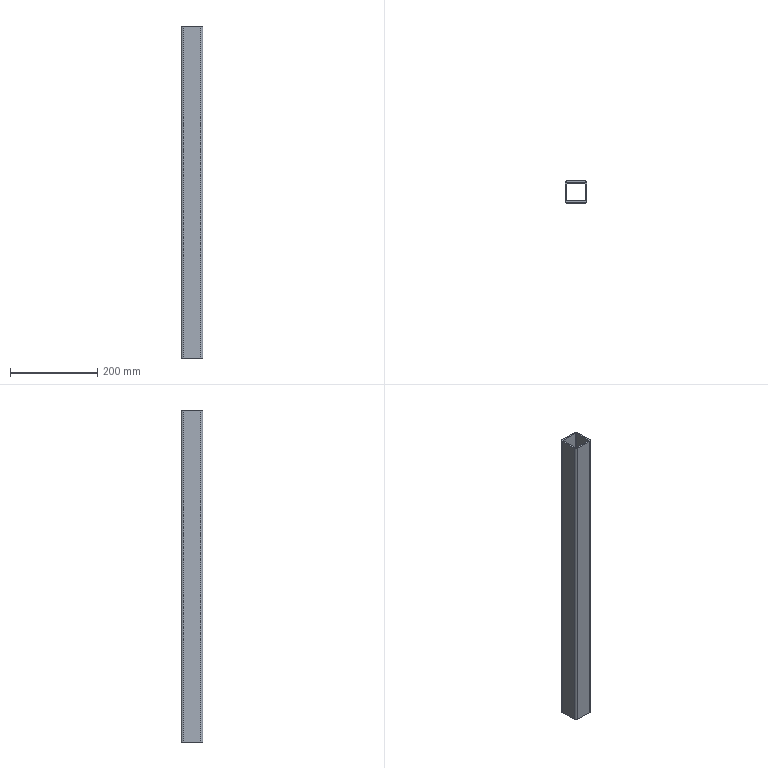Part | STEP file | 冲床-300配套压波_id1134_x_t | 1 solid | 18 faces | box 50 x 50 x 760 mm | volume 543703 mm3 | plane 10 | cylinder 8 | commonest cylinder face diameters 2 x4 10 x4
STEP:
#1=CARTESIAN_POINT('',(1164.,275.,-20.));
#2=VERTEX_POINT('',#1);
#3=CARTESIAN_POINT('',(1164.,235.,-20.));
#4=VERTEX_POINT('',#3);
#5=CARTESIAN_POINT('',(1164.,30.,-20.));
#6=DIRECTION('',(0.,-1.,0.));
#7=VECTOR('',#6,1.);
#8=LINE('',#5,#7);
#9=EDGE_CURVE('',#2,#4,#8,.T.);
#10=ORIENTED_EDGE('',*,*,#9,.F.);
#11=CARTESIAN_POINT('',(1165.,276.,-20.));
#12=VERTEX_POINT('',#11);
#13=CARTESIAN_POINT('',(1165.,275.,-20.));
#14=DIRECTION('',(0.,0.,1.));
#15=DIRECTION('',(1.,0.,0.));
#16=AXIS2_PLACEMENT_3D('',#13,#14,#15);
#17=CIRCLE('',#16,1.);
#18=EDGE_CURVE('',#12,#2,#17,.T.);
#19=ORIENTED_EDGE('',*,*,#18,.F.);
#20=CARTESIAN_POINT('',(1205.,276.,-20.));
#21=VERTEX_POINT('',#20);
#22=CARTESIAN_POINT('',(10.,276.,-20.));
#23=DIRECTION('',(-1.,0.,0.));
#24=VECTOR('',#23,1.);
#25=LINE('',#22,#24);
#26=EDGE_CURVE('',#21,#12,#25,.T.);
#27=ORIENTED_EDGE('',*,*,#26,.F.);
#28=CARTESIAN_POINT('',(1206.,275.,-20.));
#29=VERTEX_POINT('',#28);
#30=CARTESIAN_POINT('',(1205.,275.,-20.));
#31=DIRECTION('',(0.,0.,1.));
#32=DIRECTION('',(1.,0.,0.));
#33=AXIS2_PLACEMENT_3D('',#30,#31,#32);
#34=CIRCLE('',#33,1.);
#35=EDGE_CURVE('',#29,#21,#34,.T.);
#36=ORIENTED_EDGE('',*,*,#35,.F.);
#37=CARTESIAN_POINT('',(1206.,235.,-20.));
#38=VERTEX_POINT('',#37);
#39=CARTESIAN_POINT('',(1206.,30.,-20.));
#40=DIRECTION('',(0.,1.,0.));
#41=VECTOR('',#40,1.);
#42=LINE('',#39,#41);
#43=EDGE_CURVE('',#38,#29,#42,.T.);
#44=ORIENTED_EDGE('',*,*,#43,.F.);
#45=CARTESIAN_POINT('',(1205.,234.,-20.));
#46=VERTEX_POINT('',#45);
#47=CARTESIAN_POINT('',(1205.,235.,-20.));
#48=DIRECTION('',(0.,0.,1.));
#49=DIRECTION('',(1.,0.,0.));
#50=AXIS2_PLACEMENT_3D('',#47,#48,#49);
#51=CIRCLE('',#50,1.);
#52=EDGE_CURVE('',#46,#38,#51,.T.);
#53=ORIENTED_EDGE('',*,*,#52,.F.);
#54=CARTESIAN_POINT('',(1165.,234.,-20.));
#55=VERTEX_POINT('',#54);
#56=CARTESIAN_POINT('',(10.,234.,-20.));
#57=DIRECTION('',(1.,0.,0.));
#58=VECTOR('',#57,1.);
#59=LINE('',#56,#58);
#60=EDGE_CURVE('',#55,#46,#59,.T.);
#61=ORIENTED_EDGE('',*,*,#60,.F.);
#62=CARTESIAN_POINT('',(1165.,235.,-20.));
#63=DIRECTION('',(0.,0.,1.));
#64=DIRECTION('',(1.,0.,0.));
#65=AXIS2_PLACEMENT_3D('',#62,#63,#64);
#66=CIRCLE('',#65,1.);
#67=EDGE_CURVE('',#4,#55,#66,.T.);
#68=ORIENTED_EDGE('',*,*,#67,.F.);
#69=EDGE_LOOP('',(#10,#19,#27,#36,#44,#53,#61,#68));
#70=FACE_BOUND('',#69,.T.);
#71=CARTESIAN_POINT('',(1160.,275.,-20.));
#72=VERTEX_POINT('',#71);
#73=CARTESIAN_POINT('',(1160.,235.,-20.));
#74=VERTEX_POINT('',#73);
#75=CARTESIAN_POINT('',(1160.,275.,-20.));
#76=DIRECTION('',(0.,-1.,0.));
#77=VECTOR('',#76,1.);
#78=LINE('',#75,#77);
#79=EDGE_CURVE('',#72,#74,#78,.T.);
#80=ORIENTED_EDGE('',*,*,#79,.T.);
#81=CARTESIAN_POINT('',(1165.,230.,-20.));
#82=VERTEX_POINT('',#81);
#83=CARTESIAN_POINT('',(1165.,235.,-20.));
#84=DIRECTION('',(0.,0.,1.));
#85=DIRECTION('',(1.,0.,0.));
#86=AXIS2_PLACEMENT_3D('',#83,#84,#85);
#87=CIRCLE('',#86,5.);
#88=EDGE_CURVE('',#74,#82,#87,.T.);
#89=ORIENTED_EDGE('',*,*,#88,.T.);
#90=CARTESIAN_POINT('',(1205.,230.,-20.));
#91=VERTEX_POINT('',#90);
#92=CARTESIAN_POINT('',(1165.,230.,-20.));
#93=DIRECTION('',(1.,0.,0.));
#94=VECTOR('',#93,1.);
#95=LINE('',#92,#94);
#96=EDGE_CURVE('',#82,#91,#95,.T.);
#97=ORIENTED_EDGE('',*,*,#96,.T.);
#98=CARTESIAN_POINT('',(1210.,235.,-20.));
#99=VERTEX_POINT('',#98);
#100=CARTESIAN_POINT('',(1205.,235.,-20.));
#101=DIRECTION('',(0.,0.,1.));
#102=DIRECTION('',(1.,0.,0.));
#103=AXIS2_PLACEMENT_3D('',#100,#101,#102);
#104=CIRCLE('',#103,5.);
#105=EDGE_CURVE('',#91,#99,#104,.T.);
#106=ORIENTED_EDGE('',*,*,#105,.T.);
#107=CARTESIAN_POINT('',(1210.,275.,-20.));
#108=VERTEX_POINT('',#107);
#109=CARTESIAN_POINT('',(1210.,235.,-20.));
#110=DIRECTION('',(0.,1.,0.));
#111=VECTOR('',#110,1.);
#112=LINE('',#109,#111);
#113=EDGE_CURVE('',#99,#108,#112,.T.);
#114=ORIENTED_EDGE('',*,*,#113,.T.);
#115=CARTESIAN_POINT('',(1205.,280.,-20.));
#116=VERTEX_POINT('',#115);
#117=CARTESIAN_POINT('',(1205.,275.,-20.));
#118=DIRECTION('',(0.,0.,1.));
#119=DIRECTION('',(1.,0.,0.));
#120=AXIS2_PLACEMENT_3D('',#117,#118,#119);
#121=CIRCLE('',#120,5.);
#122=EDGE_CURVE('',#108,#116,#121,.T.);
#123=ORIENTED_EDGE('',*,*,#122,.T.);
#124=CARTESIAN_POINT('',(1165.,280.,-20.));
#125=VERTEX_POINT('',#124);
#126=CARTESIAN_POINT('',(1205.,280.,-20.));
#127=DIRECTION('',(-1.,0.,0.));
#128=VECTOR('',#127,1.);
#129=LINE('',#126,#128);
#130=EDGE_CURVE('',#116,#125,#129,.T.);
#131=ORIENTED_EDGE('',*,*,#130,.T.);
#132=CARTESIAN_POINT('',(1165.,275.,-20.));
#133=DIRECTION('',(0.,0.,1.));
#134=DIRECTION('',(1.,0.,0.));
#135=AXIS2_PLACEMENT_3D('',#132,#133,#134);
#136=CIRCLE('',#135,5.);
#137=EDGE_CURVE('',#125,#72,#136,.T.);
#138=ORIENTED_EDGE('',*,*,#137,.T.);
#139=EDGE_LOOP('',(#80,#89,#97,#106,#114,#123,#131,#138));
#140=FACE_BOUND('',#139,.T.);
#141=CARTESIAN_POINT('',(10.,30.,-20.));
#142=DIRECTION('',(0.,0.,1.));
#143=DIRECTION('',(1.,0.,0.));
#144=AXIS2_PLACEMENT_3D('',#141,#142,#143);
#145=PLANE('',#144);
#146=ADVANCED_FACE('',(#70,#140),#145,.T.);
#147=CARTESIAN_POINT('',(1165.,230.,-780.));
#148=VERTEX_POINT('',#147);
#149=CARTESIAN_POINT('',(1165.,230.,-740.));
#150=DIRECTION('',(0.,0.,1.));
#151=VECTOR('',#150,1.);
#152=LINE('',#149,#151);
#153=EDGE_CURVE('',#148,#82,#152,.T.);
#154=ORIENTED_EDGE('',*,*,#153,.T.);
#155=ORIENTED_EDGE('',*,*,#88,.F.);
#156=CARTESIAN_POINT('',(1160.,235.,-780.));
#157=VERTEX_POINT('',#156);
#158=CARTESIAN_POINT('',(1160.,235.,-740.));
#159=DIRECTION('',(0.,0.,1.));
#160=VECTOR('',#159,1.);
#161=LINE('',#158,#160);
#162=EDGE_CURVE('',#157,#74,#161,.T.);
#163=ORIENTED_EDGE('',*,*,#162,.F.);
#164=CARTESIAN_POINT('',(1165.,235.,-780.));
#165=DIRECTION('',(0.,0.,1.));
#166=DIRECTION('',(1.,0.,0.));
#167=AXIS2_PLACEMENT_3D('',#164,#165,#166);
#168=CIRCLE('',#167,5.);
#169=EDGE_CURVE('',#157,#148,#168,.T.);
#170=ORIENTED_EDGE('',*,*,#169,.T.);
#171=EDGE_LOOP('',(#154,#155,#163,#170));
#172=FACE_OUTER_BOUND('',#171,.T.);
#173=CARTESIAN_POINT('',(1165.,235.,-740.));
#174=DIRECTION('',(0.,0.,1.));
#175=DIRECTION('',(1.,0.,0.));
#176=AXIS2_PLACEMENT_3D('',#173,#174,#175);
#177=CYLINDRICAL_SURFACE('',#176,5.);
#178=ADVANCED_FACE('',(#172),#177,.T.);
#179=CARTESIAN_POINT('',(1205.,230.,-780.));
#180=VERTEX_POINT('',#179);
#181=CARTESIAN_POINT('',(1205.,230.,-740.));
#182=DIRECTION('',(0.,0.,1.));
#183=VECTOR('',#182,1.);
#184=LINE('',#181,#183);
#185=EDGE_CURVE('',#180,#91,#184,.T.);
#186=ORIENTED_EDGE('',*,*,#185,.T.);
#187=ORIENTED_EDGE('',*,*,#96,.F.);
#188=ORIENTED_EDGE('',*,*,#153,.F.);
#189=CARTESIAN_POINT('',(1165.,230.,-780.));
#190=DIRECTION('',(1.,0.,0.));
#191=VECTOR('',#190,1.);
#192=LINE('',#189,#191);
#193=EDGE_CURVE('',#148,#180,#192,.T.);
#194=ORIENTED_EDGE('',*,*,#193,.T.);
#195=EDGE_LOOP('',(#186,#187,#188,#194));
#196=FACE_OUTER_BOUND('',#195,.T.);
#197=CARTESIAN_POINT('',(1165.,230.,-740.));
#198=DIRECTION('',(0.,-1.,0.));
#199=DIRECTION('',(1.,0.,0.));
#200=AXIS2_PLACEMENT_3D('',#197,#198,#199);
#201=PLANE('',#200);
#202=ADVANCED_FACE('',(#196),#201,.T.);
#203=CARTESIAN_POINT('',(1210.,235.,-780.));
#204=VERTEX_POINT('',#203);
#205=CARTESIAN_POINT('',(1210.,235.,-740.));
#206=DIRECTION('',(0.,0.,1.));
#207=VECTOR('',#206,1.);
#208=LINE('',#205,#207);
#209=EDGE_CURVE('',#204,#99,#208,.T.);
#210=ORIENTED_EDGE('',*,*,#209,.T.);
#211=ORIENTED_EDGE('',*,*,#105,.F.);
#212=ORIENTED_EDGE('',*,*,#185,.F.);
#213=CARTESIAN_POINT('',(1205.,235.,-780.));
#214=DIRECTION('',(0.,0.,1.));
#215=DIRECTION('',(1.,0.,0.));
#216=AXIS2_PLACEMENT_3D('',#213,#214,#215);
#217=CIRCLE('',#216,5.);
#218=EDGE_CURVE('',#180,#204,#217,.T.);
#219=ORIENTED_EDGE('',*,*,#218,.T.);
#220=EDGE_LOOP('',(#210,#211,#212,#219));
#221=FACE_OUTER_BOUND('',#220,.T.);
#222=CARTESIAN_POINT('',(1205.,235.,-740.));
#223=DIRECTION('',(0.,0.,1.));
#224=DIRECTION('',(1.,0.,0.));
#225=AXIS2_PLACEMENT_3D('',#222,#223,#224);
#226=CYLINDRICAL_SURFACE('',#225,5.);
#227=ADVANCED_FACE('',(#221),#226,.T.);
#228=CARTESIAN_POINT('',(1210.,275.,-780.));
#229=VERTEX_POINT('',#228);
#230=CARTESIAN_POINT('',(1210.,275.,-740.));
#231=DIRECTION('',(0.,0.,1.));
#232=VECTOR('',#231,1.);
#233=LINE('',#230,#232);
#234=EDGE_CURVE('',#229,#108,#233,.T.);
#235=ORIENTED_EDGE('',*,*,#234,.T.);
#236=ORIENTED_EDGE('',*,*,#113,.F.);
#237=ORIENTED_EDGE('',*,*,#209,.F.);
#238=CARTESIAN_POINT('',(1210.,235.,-780.));
#239=DIRECTION('',(0.,1.,0.));
#240=VECTOR('',#239,1.);
#241=LINE('',#238,#240);
#242=EDGE_CURVE('',#204,#229,#241,.T.);
#243=ORIENTED_EDGE('',*,*,#242,.T.);
#244=EDGE_LOOP('',(#235,#236,#237,#243));
#245=FACE_OUTER_BOUND('',#244,.T.);
#246=CARTESIAN_POINT('',(1210.,235.,-740.));
#247=DIRECTION('',(1.,0.,0.));
#248=DIRECTION('',(0.,0.,-1.));
#249=AXIS2_PLACEMENT_3D('',#246,#247,#248);
#250=PLANE('',#249);
#251=ADVANCED_FACE('',(#245),#250,.T.);
#252=CARTESIAN_POINT('',(1205.,280.,-780.));
#253=VERTEX_POINT('',#252);
#254=CARTESIAN_POINT('',(1205.,280.,-740.));
#255=DIRECTION('',(0.,0.,1.));
#256=VECTOR('',#255,1.);
#257=LINE('',#254,#256);
#258=EDGE_CURVE('',#253,#116,#257,.T.);
#259=ORIENTED_EDGE('',*,*,#258,.T.);
#260=ORIENTED_EDGE('',*,*,#122,.F.);
#261=ORIENTED_EDGE('',*,*,#234,.F.);
#262=CARTESIAN_POINT('',(1205.,275.,-780.));
#263=DIRECTION('',(0.,0.,1.));
#264=DIRECTION('',(1.,0.,0.));
#265=AXIS2_PLACEMENT_3D('',#262,#263,#264);
#266=CIRCLE('',#265,5.);
#267=EDGE_CURVE('',#229,#253,#266,.T.);
#268=ORIENTED_EDGE('',*,*,#267,.T.);
#269=EDGE_LOOP('',(#259,#260,#261,#268));
#270=FACE_OUTER_BOUND('',#269,.T.);
#271=CARTESIAN_POINT('',(1205.,275.,-740.));
#272=DIRECTION('',(0.,0.,1.));
#273=DIRECTION('',(1.,0.,0.));
#274=AXIS2_PLACEMENT_3D('',#271,#272,#273);
#275=CYLINDRICAL_SURFACE('',#274,5.);
#276=ADVANCED_FACE('',(#270),#275,.T.);
#277=CARTESIAN_POINT('',(1165.,276.,-780.));
#278=VERTEX_POINT('',#277);
#279=CARTESIAN_POINT('',(1164.,275.,-780.));
#280=VERTEX_POINT('',#279);
#281=CARTESIAN_POINT('',(1165.,275.,-780.));
#282=DIRECTION('',(0.,0.,1.));
#283=DIRECTION('',(1.,0.,0.));
#284=AXIS2_PLACEMENT_3D('',#281,#282,#283);
#285=CIRCLE('',#284,1.);
#286=EDGE_CURVE('',#278,#280,#285,.T.);
#287=ORIENTED_EDGE('',*,*,#286,.T.);
#288=CARTESIAN_POINT('',(1164.,235.,-780.));
#289=VERTEX_POINT('',#288);
#290=CARTESIAN_POINT('',(1164.,235.,-780.));
#291=DIRECTION('',(0.,-1.,0.));
#292=VECTOR('',#291,1.);
#293=LINE('',#290,#292);
#294=EDGE_CURVE('',#280,#289,#293,.T.);
#295=ORIENTED_EDGE('',*,*,#294,.T.);
#296=CARTESIAN_POINT('',(1165.,234.,-780.));
#297=VERTEX_POINT('',#296);
#298=CARTESIAN_POINT('',(1165.,235.,-780.));
#299=DIRECTION('',(0.,0.,1.));
#300=DIRECTION('',(1.,0.,0.));
#301=AXIS2_PLACEMENT_3D('',#298,#299,#300);
#302=CIRCLE('',#301,1.);
#303=EDGE_CURVE('',#289,#297,#302,.T.);
#304=ORIENTED_EDGE('',*,*,#303,.T.);
#305=CARTESIAN_POINT('',(1205.,234.,-780.));
#306=VERTEX_POINT('',#305);
#307=CARTESIAN_POINT('',(1165.,234.,-780.));
#308=DIRECTION('',(1.,0.,0.));
#309=VECTOR('',#308,1.);
#310=LINE('',#307,#309);
#311=EDGE_CURVE('',#297,#306,#310,.T.);
#312=ORIENTED_EDGE('',*,*,#311,.T.);
#313=CARTESIAN_POINT('',(1206.,235.,-780.));
#314=VERTEX_POINT('',#313);
#315=CARTESIAN_POINT('',(1205.,235.,-780.));
#316=DIRECTION('',(0.,0.,1.));
#317=DIRECTION('',(1.,0.,0.));
#318=AXIS2_PLACEMENT_3D('',#315,#316,#317);
#319=CIRCLE('',#318,1.);
#320=EDGE_CURVE('',#306,#314,#319,.T.);
#321=ORIENTED_EDGE('',*,*,#320,.T.);
#322=CARTESIAN_POINT('',(1206.,275.,-780.));
#323=VERTEX_POINT('',#322);
#324=CARTESIAN_POINT('',(1206.,235.,-780.));
#325=DIRECTION('',(0.,1.,0.));
#326=VECTOR('',#325,1.);
#327=LINE('',#324,#326);
#328=EDGE_CURVE('',#314,#323,#327,.T.);
#329=ORIENTED_EDGE('',*,*,#328,.T.);
#330=CARTESIAN_POINT('',(1205.,276.,-780.));
#331=VERTEX_POINT('',#330);
#332=CARTESIAN_POINT('',(1205.,275.,-780.));
#333=DIRECTION('',(0.,0.,1.));
#334=DIRECTION('',(1.,0.,0.));
#335=AXIS2_PLACEMENT_3D('',#332,#333,#334);
#336=CIRCLE('',#335,1.);
#337=EDGE_CURVE('',#323,#331,#336,.T.);
#338=ORIENTED_EDGE('',*,*,#337,.T.);
#339=CARTESIAN_POINT('',(1165.,276.,-780.));
#340=DIRECTION('',(-1.,0.,0.));
#341=VECTOR('',#340,1.);
#342=LINE('',#339,#341);
#343=EDGE_CURVE('',#331,#278,#342,.T.);
#344=ORIENTED_EDGE('',*,*,#343,.T.);
#345=EDGE_LOOP('',(#287,#295,#304,#312,#321,#329,#338,#344));
#346=FACE_BOUND('',#345,.T.);
#347=CARTESIAN_POINT('',(1160.,275.,-780.));
#348=VERTEX_POINT('',#347);
#349=CARTESIAN_POINT('',(1160.,235.,-780.));
#350=DIRECTION('',(0.,-1.,0.));
#351=VECTOR('',#350,1.);
#352=LINE('',#349,#351);
#353=EDGE_CURVE('',#348,#157,#352,.T.);
#354=ORIENTED_EDGE('',*,*,#353,.F.);
#355=CARTESIAN_POINT('',(1165.,280.,-780.));
#356=VERTEX_POINT('',#355);
#357=CARTESIAN_POINT('',(1165.,275.,-780.));
#358=DIRECTION('',(0.,0.,1.));
#359=DIRECTION('',(1.,0.,0.));
#360=AXIS2_PLACEMENT_3D('',#357,#358,#359);
#361=CIRCLE('',#360,5.);
#362=EDGE_CURVE('',#356,#348,#361,.T.);
#363=ORIENTED_EDGE('',*,*,#362,.F.);
#364=CARTESIAN_POINT('',(1165.,280.,-780.));
#365=DIRECTION('',(-1.,0.,0.));
#366=VECTOR('',#365,1.);
#367=LINE('',#364,#366);
#368=EDGE_CURVE('',#253,#356,#367,.T.);
#369=ORIENTED_EDGE('',*,*,#368,.F.);
#370=ORIENTED_EDGE('',*,*,#267,.F.);
#371=ORIENTED_EDGE('',*,*,#242,.F.);
#372=ORIENTED_EDGE('',*,*,#218,.F.);
#373=ORIENTED_EDGE('',*,*,#193,.F.);
#374=ORIENTED_EDGE('',*,*,#169,.F.);
#375=EDGE_LOOP('',(#354,#363,#369,#370,#371,#372,#373,#374));
#376=FACE_BOUND('',#375,.T.);
#377=CARTESIAN_POINT('',(1165.,235.,-780.));
#378=DIRECTION('',(0.,0.,1.));
#379=DIRECTION('',(1.,0.,0.));
#380=AXIS2_PLACEMENT_3D('',#377,#378,#379);
#381=PLANE('',#380);
#382=ADVANCED_FACE('',(#346,#376),#381,.F.);
#383=CARTESIAN_POINT('',(1165.,280.,-740.));
#384=DIRECTION('',(0.,0.,1.));
#385=VECTOR('',#384,1.);
#386=LINE('',#383,#385);
#387=EDGE_CURVE('',#356,#125,#386,.T.);
#388=ORIENTED_EDGE('',*,*,#387,.T.);
#389=ORIENTED_EDGE('',*,*,#130,.F.);
#390=ORIENTED_EDGE('',*,*,#258,.F.);
#391=ORIENTED_EDGE('',*,*,#368,.T.);
#392=EDGE_LOOP('',(#388,#389,#390,#391));
#393=FACE_OUTER_BOUND('',#392,.T.);
#394=CARTESIAN_POINT('',(1205.,280.,-740.));
#395=DIRECTION('',(0.,1.,0.));
#396=DIRECTION('',(-1.,0.,0.));
#397=AXIS2_PLACEMENT_3D('',#394,#395,#396);
#398=PLANE('',#397);
#399=ADVANCED_FACE('',(#393),#398,.T.);
#400=ORIENTED_EDGE('',*,*,#162,.T.);
#401=ORIENTED_EDGE('',*,*,#79,.F.);
#402=CARTESIAN_POINT('',(1160.,275.,-740.));
#403=DIRECTION('',(0.,0.,1.));
#404=VECTOR('',#403,1.);
#405=LINE('',#402,#404);
#406=EDGE_CURVE('',#348,#72,#405,.T.);
#407=ORIENTED_EDGE('',*,*,#406,.F.);
#408=ORIENTED_EDGE('',*,*,#353,.T.);
#409=EDGE_LOOP('',(#400,#401,#407,#408));
#410=FACE_OUTER_BOUND('',#409,.T.);
#411=CARTESIAN_POINT('',(1160.,275.,-740.));
#412=DIRECTION('',(-1.,0.,0.));
#413=DIRECTION('',(0.,0.,1.));
#414=AXIS2_PLACEMENT_3D('',#411,#412,#413);
#415=PLANE('',#414);
#416=ADVANCED_FACE('',(#410),#415,.T.);
#417=ORIENTED_EDGE('',*,*,#406,.T.);
#418=ORIENTED_EDGE('',*,*,#137,.F.);
#419=ORIENTED_EDGE('',*,*,#387,.F.);
#420=ORIENTED_EDGE('',*,*,#362,.T.);
#421=EDGE_LOOP('',(#417,#418,#419,#420));
#422=FACE_OUTER_BOUND('',#421,.T.);
#423=CARTESIAN_POINT('',(1165.,275.,-740.));
#424=DIRECTION('',(0.,0.,1.));
#425=DIRECTION('',(1.,0.,0.));
#426=AXIS2_PLACEMENT_3D('',#423,#424,#425);
#427=CYLINDRICAL_SURFACE('',#426,5.);
#428=ADVANCED_FACE('',(#422),#427,.T.);
#429=CARTESIAN_POINT('',(1165.,234.,-740.));
#430=DIRECTION('',(0.,0.,1.));
#431=VECTOR('',#430,1.);
#432=LINE('',#429,#431);
#433=EDGE_CURVE('',#297,#55,#432,.T.);
#434=ORIENTED_EDGE('',*,*,#433,.F.);
#435=ORIENTED_EDGE('',*,*,#303,.F.);
#436=CARTESIAN_POINT('',(1164.,235.,-740.));
#437=DIRECTION('',(0.,0.,1.));
#438=VECTOR('',#437,1.);
#439=LINE('',#436,#438);
#440=EDGE_CURVE('',#289,#4,#439,.T.);
#441=ORIENTED_EDGE('',*,*,#440,.T.);
#442=ORIENTED_EDGE('',*,*,#67,.T.);
#443=EDGE_LOOP('',(#434,#435,#441,#442));
#444=FACE_OUTER_BOUND('',#443,.T.);
#445=CARTESIAN_POINT('',(1165.,235.,-740.));
#446=DIRECTION('',(0.,0.,1.));
#447=DIRECTION('',(1.,0.,0.));
#448=AXIS2_PLACEMENT_3D('',#445,#446,#447);
#449=CYLINDRICAL_SURFACE('',#448,1.);
#450=ADVANCED_FACE('',(#444),#449,.F.);
#451=CARTESIAN_POINT('',(1205.,234.,-740.));
#452=DIRECTION('',(0.,0.,1.));
#453=VECTOR('',#452,1.);
#454=LINE('',#451,#453);
#455=EDGE_CURVE('',#306,#46,#454,.T.);
#456=ORIENTED_EDGE('',*,*,#455,.F.);
#457=ORIENTED_EDGE('',*,*,#311,.F.);
#458=ORIENTED_EDGE('',*,*,#433,.T.);
#459=ORIENTED_EDGE('',*,*,#60,.T.);
#460=EDGE_LOOP('',(#456,#457,#458,#459));
#461=FACE_OUTER_BOUND('',#460,.T.);
#462=CARTESIAN_POINT('',(1165.,234.,-740.));
#463=DIRECTION('',(0.,-1.,0.));
#464=DIRECTION('',(1.,0.,0.));
#465=AXIS2_PLACEMENT_3D('',#462,#463,#464);
#466=PLANE('',#465);
#467=ADVANCED_FACE('',(#461),#466,.F.);
#468=CARTESIAN_POINT('',(1206.,235.,-740.));
#469=DIRECTION('',(0.,0.,1.));
#470=VECTOR('',#469,1.);
#471=LINE('',#468,#470);
#472=EDGE_CURVE('',#314,#38,#471,.T.);
#473=ORIENTED_EDGE('',*,*,#472,.F.);
#474=ORIENTED_EDGE('',*,*,#320,.F.);
#475=ORIENTED_EDGE('',*,*,#455,.T.);
#476=ORIENTED_EDGE('',*,*,#52,.T.);
#477=EDGE_LOOP('',(#473,#474,#475,#476));
#478=FACE_OUTER_BOUND('',#477,.T.);
#479=CARTESIAN_POINT('',(1205.,235.,-740.));
#480=DIRECTION('',(0.,0.,1.));
#481=DIRECTION('',(1.,0.,0.));
#482=AXIS2_PLACEMENT_3D('',#479,#480,#481);
#483=CYLINDRICAL_SURFACE('',#482,1.);
#484=ADVANCED_FACE('',(#478),#483,.F.);
#485=CARTESIAN_POINT('',(1206.,275.,-740.));
#486=DIRECTION('',(0.,0.,1.));
#487=VECTOR('',#486,1.);
#488=LINE('',#485,#487);
#489=EDGE_CURVE('',#323,#29,#488,.T.);
#490=ORIENTED_EDGE('',*,*,#489,.F.);
#491=ORIENTED_EDGE('',*,*,#328,.F.);
#492=ORIENTED_EDGE('',*,*,#472,.T.);
#493=ORIENTED_EDGE('',*,*,#43,.T.);
#494=EDGE_LOOP('',(#490,#491,#492,#493));
#495=FACE_OUTER_BOUND('',#494,.T.);
#496=CARTESIAN_POINT('',(1206.,235.,-740.));
#497=DIRECTION('',(1.,0.,0.));
#498=DIRECTION('',(0.,0.,-1.));
#499=AXIS2_PLACEMENT_3D('',#496,#497,#498);
#500=PLANE('',#499);
#501=ADVANCED_FACE('',(#495),#500,.F.);
#502=CARTESIAN_POINT('',(1205.,276.,-740.));
#503=DIRECTION('',(0.,0.,1.));
#504=VECTOR('',#503,1.);
#505=LINE('',#502,#504);
#506=EDGE_CURVE('',#331,#21,#505,.T.);
#507=ORIENTED_EDGE('',*,*,#506,.F.);
#508=ORIENTED_EDGE('',*,*,#337,.F.);
#509=ORIENTED_EDGE('',*,*,#489,.T.);
#510=ORIENTED_EDGE('',*,*,#35,.T.);
#511=EDGE_LOOP('',(#507,#508,#509,#510));
#512=FACE_OUTER_BOUND('',#511,.T.);
#513=CARTESIAN_POINT('',(1205.,275.,-740.));
#514=DIRECTION('',(0.,0.,1.));
#515=DIRECTION('',(1.,0.,0.));
#516=AXIS2_PLACEMENT_3D('',#513,#514,#515);
#517=CYLINDRICAL_SURFACE('',#516,1.);
#518=ADVANCED_FACE('',(#512),#517,.F.);
#519=CARTESIAN_POINT('',(1165.,276.,-740.));
#520=DIRECTION('',(0.,0.,1.));
#521=VECTOR('',#520,1.);
#522=LINE('',#519,#521);
#523=EDGE_CURVE('',#278,#12,#522,.T.);
#524=ORIENTED_EDGE('',*,*,#523,.F.);
#525=ORIENTED_EDGE('',*,*,#343,.F.);
#526=ORIENTED_EDGE('',*,*,#506,.T.);
#527=ORIENTED_EDGE('',*,*,#26,.T.);
#528=EDGE_LOOP('',(#524,#525,#526,#527));
#529=FACE_OUTER_BOUND('',#528,.T.);
#530=CARTESIAN_POINT('',(1205.,276.,-740.));
#531=DIRECTION('',(0.,1.,0.));
#532=DIRECTION('',(-1.,0.,0.));
#533=AXIS2_PLACEMENT_3D('',#530,#531,#532);
#534=PLANE('',#533);
#535=ADVANCED_FACE('',(#529),#534,.F.);
#536=ORIENTED_EDGE('',*,*,#440,.F.);
#537=ORIENTED_EDGE('',*,*,#294,.F.);
#538=CARTESIAN_POINT('',(1164.,275.,-740.));
#539=DIRECTION('',(0.,0.,1.));
#540=VECTOR('',#539,1.);
#541=LINE('',#538,#540);
#542=EDGE_CURVE('',#280,#2,#541,.T.);
#543=ORIENTED_EDGE('',*,*,#542,.T.);
#544=ORIENTED_EDGE('',*,*,#9,.T.);
#545=EDGE_LOOP('',(#536,#537,#543,#544));
#546=FACE_OUTER_BOUND('',#545,.T.);
#547=CARTESIAN_POINT('',(1164.,275.,-740.));
#548=DIRECTION('',(-1.,0.,0.));
#549=DIRECTION('',(0.,0.,1.));
#550=AXIS2_PLACEMENT_3D('',#547,#548,#549);
#551=PLANE('',#550);
#552=ADVANCED_FACE('',(#546),#551,.F.);
#553=ORIENTED_EDGE('',*,*,#542,.F.);
#554=ORIENTED_EDGE('',*,*,#286,.F.);
#555=ORIENTED_EDGE('',*,*,#523,.T.);
#556=ORIENTED_EDGE('',*,*,#18,.T.);
#557=EDGE_LOOP('',(#553,#554,#555,#556));
#558=FACE_OUTER_BOUND('',#557,.T.);
#559=CARTESIAN_POINT('',(1165.,275.,-740.));
#560=DIRECTION('',(0.,0.,1.));
#561=DIRECTION('',(1.,0.,0.));
#562=AXIS2_PLACEMENT_3D('',#559,#560,#561);
#563=CYLINDRICAL_SURFACE('',#562,1.);
#564=ADVANCED_FACE('',(#558),#563,.F.);
#565=CLOSED_SHELL('',(#146,#178,#202,#227,#251,#276,#382,#399,#416,#428,#450,#467,#484,#501,#518,#535,#552,#564));
#566=MANIFOLD_SOLID_BREP('',#565);
#567=(LENGTH_UNIT()NAMED_UNIT(*)SI_UNIT(.MILLI.,.METRE.));
#568=UNCERTAINTY_MEASURE_WITH_UNIT(LENGTH_MEASURE(0.00002),#567,'','');
#569=(NAMED_UNIT(*)PLANE_ANGLE_UNIT()SI_UNIT($,.RADIAN.));
#570=PLANE_ANGLE_MEASURE_WITH_UNIT(PLANE_ANGLE_MEASURE(0.01745),#569);
#571=DIMENSIONAL_EXPONENTS(0.,0.,0.,0.,0.,0.,0.);
#572=(CONVERSION_BASED_UNIT('DEGREE',#570)NAMED_UNIT(#571)PLANE_ANGLE_UNIT());
#573=(NAMED_UNIT(*)SI_UNIT($,.STERADIAN.)SOLID_ANGLE_UNIT());
#574=(GEOMETRIC_REPRESENTATION_CONTEXT(3)GLOBAL_UNCERTAINTY_ASSIGNED_CONTEXT((#568))GLOBAL_UNIT_ASSIGNED_CONTEXT((#567,#572,#573))REPRESENTATION_CONTEXT('',''));
#575=ADVANCED_BREP_SHAPE_REPRESENTATION('',(#566),#574);